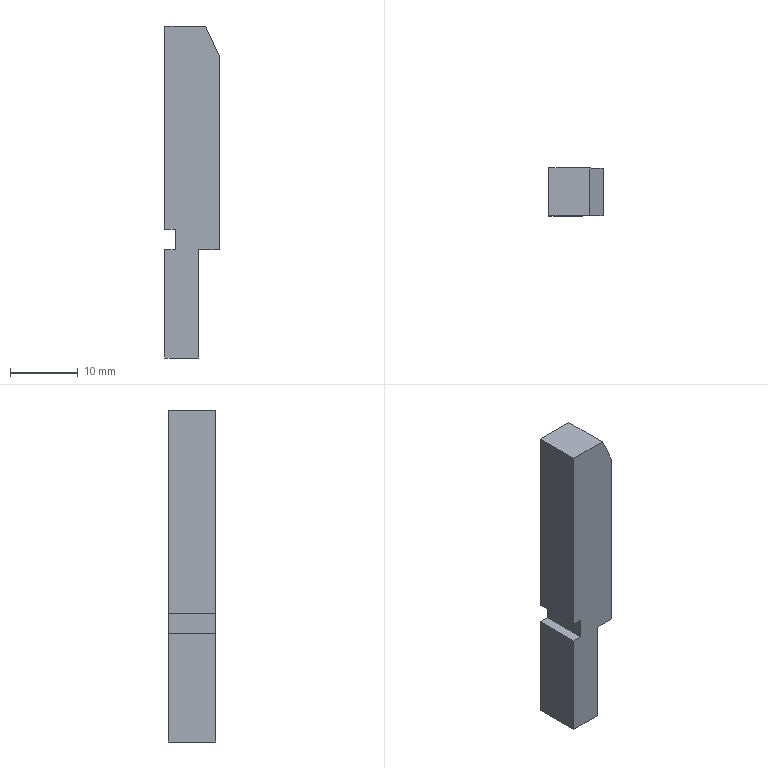Part | STEP file | Riveting product locating pin | 1 solid | 13 faces | box 8 x 7 x 49 mm | volume 2346 mm3 | plane 13
STEP:
#1=CARTESIAN_POINT('',(0.,0.,0.));
#2=DIRECTION('',(0.,0.,1.));
#3=DIRECTION('',(1.,0.,0.));
#4=AXIS2_PLACEMENT_3D('',#1,#2,#3);
#5=CARTESIAN_POINT('',(0.,8.,49.));
#6=VERTEX_POINT('',#5);
#7=CARTESIAN_POINT('',(0.,8.,19.));
#8=VERTEX_POINT('',#7);
#9=CARTESIAN_POINT('',(0.,8.,49.));
#10=DIRECTION('',(0.,0.,-1.));
#11=VECTOR('',#10,1.);
#12=LINE('',#9,#11);
#13=CARTESIAN_POINT('',(0.,0.,49.));
#14=DIRECTION('',(1.,0.,0.));
#15=DIRECTION('',(0.,0.,-1.));
#16=AXIS2_PLACEMENT_3D('',#13,#14,#15);
#17=PLANE('',#16);
#18=CARTESIAN_POINT('',(0.,8.));
#19=DIRECTION('',(1.,0.));
#20=VECTOR('',#19,1.);
#21=LINE('',#18,#20);
#22=(GEOMETRIC_REPRESENTATION_CONTEXT(2)PARAMETRIC_REPRESENTATION_CONTEXT()REPRESENTATION_CONTEXT('',''));
#23=DEFINITIONAL_REPRESENTATION('',(#21),#22);
#24=PCURVE('',#17,#23);
#25=CARTESIAN_POINT('',(0.,8.,49.));
#26=DIRECTION('',(0.,-1.,0.));
#27=DIRECTION('',(0.,0.,-1.));
#28=AXIS2_PLACEMENT_3D('',#25,#26,#27);
#29=PLANE('',#28);
#30=CARTESIAN_POINT('',(0.,0.));
#31=DIRECTION('',(1.,0.));
#32=VECTOR('',#31,1.);
#33=LINE('',#30,#32);
#34=(GEOMETRIC_REPRESENTATION_CONTEXT(2)PARAMETRIC_REPRESENTATION_CONTEXT()REPRESENTATION_CONTEXT('',''));
#35=DEFINITIONAL_REPRESENTATION('',(#33),#34);
#36=PCURVE('',#29,#35);
#37=SURFACE_CURVE('',#12,(#24,#36),.PCURVE_S1.);
#38=EDGE_CURVE('',#6,#8,#37,.T.);
#39=ORIENTED_EDGE('',*,*,#38,.T.);
#40=CARTESIAN_POINT('',(0.,1.,19.));
#41=VERTEX_POINT('',#40);
#42=CARTESIAN_POINT('',(0.,15.846,19.));
#43=DIRECTION('',(0.,1.,0.));
#44=VECTOR('',#43,1.);
#45=LINE('',#42,#44);
#46=CARTESIAN_POINT('',(30.,15.846));
#47=DIRECTION('',(0.,1.));
#48=VECTOR('',#47,1.);
#49=LINE('',#46,#48);
#50=(GEOMETRIC_REPRESENTATION_CONTEXT(2)PARAMETRIC_REPRESENTATION_CONTEXT()REPRESENTATION_CONTEXT('',''));
#51=DEFINITIONAL_REPRESENTATION('',(#49),#50);
#52=PCURVE('',#17,#51);
#53=CARTESIAN_POINT('',(1.5,15.846,19.));
#54=DIRECTION('',(0.,0.,1.));
#55=DIRECTION('',(0.,-1.,0.));
#56=AXIS2_PLACEMENT_3D('',#53,#54,#55);
#57=PLANE('',#56);
#58=CARTESIAN_POINT('',(0.,-1.5));
#59=DIRECTION('',(-1.,0.));
#60=VECTOR('',#59,1.);
#61=LINE('',#58,#60);
#62=(GEOMETRIC_REPRESENTATION_CONTEXT(2)PARAMETRIC_REPRESENTATION_CONTEXT()REPRESENTATION_CONTEXT('',''));
#63=DEFINITIONAL_REPRESENTATION('',(#61),#62);
#64=PCURVE('',#57,#63);
#65=SURFACE_CURVE('',#45,(#52,#64),.PCURVE_S1.);
#66=EDGE_CURVE('',#41,#8,#65,.T.);
#67=ORIENTED_EDGE('',*,*,#66,.F.);
#68=CARTESIAN_POINT('',(0.,1.,49.));
#69=VERTEX_POINT('',#68);
#70=CARTESIAN_POINT('',(0.,1.,49.));
#71=DIRECTION('',(0.,0.,-1.));
#72=VECTOR('',#71,1.);
#73=LINE('',#70,#72);
#74=CARTESIAN_POINT('',(0.,1.));
#75=DIRECTION('',(1.,0.));
#76=VECTOR('',#75,1.);
#77=LINE('',#74,#76);
#78=(GEOMETRIC_REPRESENTATION_CONTEXT(2)PARAMETRIC_REPRESENTATION_CONTEXT()REPRESENTATION_CONTEXT('',''));
#79=DEFINITIONAL_REPRESENTATION('',(#77),#78);
#80=PCURVE('',#17,#79);
#81=CARTESIAN_POINT('',(0.,1.,49.));
#82=DIRECTION('',(0.,1.,0.));
#83=DIRECTION('',(0.,0.,1.));
#84=AXIS2_PLACEMENT_3D('',#81,#82,#83);
#85=PLANE('',#84);
#86=CARTESIAN_POINT('',(0.,0.));
#87=DIRECTION('',(-1.,0.));
#88=VECTOR('',#87,1.);
#89=LINE('',#86,#88);
#90=(GEOMETRIC_REPRESENTATION_CONTEXT(2)PARAMETRIC_REPRESENTATION_CONTEXT()REPRESENTATION_CONTEXT('',''));
#91=DEFINITIONAL_REPRESENTATION('',(#89),#90);
#92=PCURVE('',#85,#91);
#93=SURFACE_CURVE('',#73,(#80,#92),.PCURVE_S1.);
#94=EDGE_CURVE('',#69,#41,#93,.T.);
#95=ORIENTED_EDGE('',*,*,#94,.F.);
#96=CARTESIAN_POINT('',(0.,0.,49.));
#97=DIRECTION('',(0.,-1.,0.));
#98=VECTOR('',#97,1.);
#99=LINE('',#96,#98);
#100=CARTESIAN_POINT('',(0.,0.));
#101=DIRECTION('',(0.,-1.));
#102=VECTOR('',#101,1.);
#103=LINE('',#100,#102);
#104=(GEOMETRIC_REPRESENTATION_CONTEXT(2)PARAMETRIC_REPRESENTATION_CONTEXT()REPRESENTATION_CONTEXT('',''));
#105=DEFINITIONAL_REPRESENTATION('',(#103),#104);
#106=PCURVE('',#17,#105);
#107=CARTESIAN_POINT('',(0.,8.,49.));
#108=DIRECTION('',(0.,0.,-1.));
#109=DIRECTION('',(-1.,0.,0.));
#110=AXIS2_PLACEMENT_3D('',#107,#108,#109);
#111=PLANE('',#110);
#112=CARTESIAN_POINT('',(0.,-8.));
#113=DIRECTION('',(0.,-1.));
#114=VECTOR('',#113,1.);
#115=LINE('',#112,#114);
#116=(GEOMETRIC_REPRESENTATION_CONTEXT(2)PARAMETRIC_REPRESENTATION_CONTEXT()REPRESENTATION_CONTEXT('',''));
#117=DEFINITIONAL_REPRESENTATION('',(#115),#116);
#118=PCURVE('',#111,#117);
#119=SURFACE_CURVE('',#99,(#106,#118),.PCURVE_S1.);
#120=EDGE_CURVE('',#6,#69,#119,.T.);
#121=ORIENTED_EDGE('',*,*,#120,.F.);
#122=EDGE_LOOP('',(#39,#67,#95,#121));
#123=FACE_BOUND('',#122,.T.);
#124=ADVANCED_FACE('',(#123),#17,.F.);
#125=CARTESIAN_POINT('',(0.,1.,16.));
#126=VERTEX_POINT('',#125);
#127=CARTESIAN_POINT('',(0.,1.,0.));
#128=VERTEX_POINT('',#127);
#129=CARTESIAN_POINT('',(0.,1.,49.));
#130=DIRECTION('',(0.,0.,-1.));
#131=VECTOR('',#130,1.);
#132=LINE('',#129,#131);
#133=CARTESIAN_POINT('',(0.,0.,49.));
#134=DIRECTION('',(1.,0.,0.));
#135=DIRECTION('',(0.,0.,-1.));
#136=AXIS2_PLACEMENT_3D('',#133,#134,#135);
#137=PLANE('',#136);
#138=CARTESIAN_POINT('',(0.,1.));
#139=DIRECTION('',(1.,0.));
#140=VECTOR('',#139,1.);
#141=LINE('',#138,#140);
#142=(GEOMETRIC_REPRESENTATION_CONTEXT(2)PARAMETRIC_REPRESENTATION_CONTEXT()REPRESENTATION_CONTEXT('',''));
#143=DEFINITIONAL_REPRESENTATION('',(#141),#142);
#144=PCURVE('',#137,#143);
#145=CARTESIAN_POINT('',(0.,0.));
#146=DIRECTION('',(-1.,0.));
#147=VECTOR('',#146,1.);
#148=LINE('',#145,#147);
#149=(GEOMETRIC_REPRESENTATION_CONTEXT(2)PARAMETRIC_REPRESENTATION_CONTEXT()REPRESENTATION_CONTEXT('',''));
#150=DEFINITIONAL_REPRESENTATION('',(#148),#149);
#151=PCURVE('',#85,#150);
#152=SURFACE_CURVE('',#132,(#144,#151),.PCURVE_S1.);
#153=EDGE_CURVE('',#126,#128,#152,.T.);
#154=ORIENTED_EDGE('',*,*,#153,.F.);
#155=CARTESIAN_POINT('',(0.,8.,16.));
#156=VERTEX_POINT('',#155);
#157=CARTESIAN_POINT('',(0.,15.846,16.));
#158=DIRECTION('',(0.,-1.,0.));
#159=VECTOR('',#158,1.);
#160=LINE('',#157,#159);
#161=CARTESIAN_POINT('',(33.,15.846));
#162=DIRECTION('',(0.,-1.));
#163=VECTOR('',#162,1.);
#164=LINE('',#161,#163);
#165=(GEOMETRIC_REPRESENTATION_CONTEXT(2)PARAMETRIC_REPRESENTATION_CONTEXT()REPRESENTATION_CONTEXT('',''));
#166=DEFINITIONAL_REPRESENTATION('',(#164),#165);
#167=PCURVE('',#137,#166);
#168=CARTESIAN_POINT('',(1.5,15.846,16.));
#169=DIRECTION('',(0.,0.,-1.));
#170=DIRECTION('',(0.,1.,0.));
#171=AXIS2_PLACEMENT_3D('',#168,#169,#170);
#172=PLANE('',#171);
#173=CARTESIAN_POINT('',(0.,-1.5));
#174=DIRECTION('',(-1.,0.));
#175=VECTOR('',#174,1.);
#176=LINE('',#173,#175);
#177=(GEOMETRIC_REPRESENTATION_CONTEXT(2)PARAMETRIC_REPRESENTATION_CONTEXT()REPRESENTATION_CONTEXT('',''));
#178=DEFINITIONAL_REPRESENTATION('',(#176),#177);
#179=PCURVE('',#172,#178);
#180=SURFACE_CURVE('',#160,(#167,#179),.PCURVE_S1.);
#181=EDGE_CURVE('',#156,#126,#180,.T.);
#182=ORIENTED_EDGE('',*,*,#181,.F.);
#183=CARTESIAN_POINT('',(0.,8.,0.));
#184=VERTEX_POINT('',#183);
#185=CARTESIAN_POINT('',(0.,8.,49.));
#186=DIRECTION('',(0.,0.,-1.));
#187=VECTOR('',#186,1.);
#188=LINE('',#185,#187);
#189=CARTESIAN_POINT('',(0.,8.));
#190=DIRECTION('',(1.,0.));
#191=VECTOR('',#190,1.);
#192=LINE('',#189,#191);
#193=(GEOMETRIC_REPRESENTATION_CONTEXT(2)PARAMETRIC_REPRESENTATION_CONTEXT()REPRESENTATION_CONTEXT('',''));
#194=DEFINITIONAL_REPRESENTATION('',(#192),#193);
#195=PCURVE('',#137,#194);
#196=CARTESIAN_POINT('',(0.,0.));
#197=DIRECTION('',(1.,0.));
#198=VECTOR('',#197,1.);
#199=LINE('',#196,#198);
#200=(GEOMETRIC_REPRESENTATION_CONTEXT(2)PARAMETRIC_REPRESENTATION_CONTEXT()REPRESENTATION_CONTEXT('',''));
#201=DEFINITIONAL_REPRESENTATION('',(#199),#200);
#202=PCURVE('',#29,#201);
#203=SURFACE_CURVE('',#188,(#195,#202),.PCURVE_S1.);
#204=EDGE_CURVE('',#156,#184,#203,.T.);
#205=ORIENTED_EDGE('',*,*,#204,.T.);
#206=CARTESIAN_POINT('',(0.,0.,0.));
#207=DIRECTION('',(0.,-1.,0.));
#208=VECTOR('',#207,1.);
#209=LINE('',#206,#208);
#210=CARTESIAN_POINT('',(49.,0.));
#211=DIRECTION('',(0.,-1.));
#212=VECTOR('',#211,1.);
#213=LINE('',#210,#212);
#214=(GEOMETRIC_REPRESENTATION_CONTEXT(2)PARAMETRIC_REPRESENTATION_CONTEXT()REPRESENTATION_CONTEXT('',''));
#215=DEFINITIONAL_REPRESENTATION('',(#213),#214);
#216=PCURVE('',#137,#215);
#217=CARTESIAN_POINT('',(0.,8.,0.));
#218=DIRECTION('',(0.,0.,-1.));
#219=DIRECTION('',(-1.,0.,0.));
#220=AXIS2_PLACEMENT_3D('',#217,#218,#219);
#221=PLANE('',#220);
#222=CARTESIAN_POINT('',(0.,-8.));
#223=DIRECTION('',(0.,-1.));
#224=VECTOR('',#223,1.);
#225=LINE('',#222,#224);
#226=(GEOMETRIC_REPRESENTATION_CONTEXT(2)PARAMETRIC_REPRESENTATION_CONTEXT()REPRESENTATION_CONTEXT('',''));
#227=DEFINITIONAL_REPRESENTATION('',(#225),#226);
#228=PCURVE('',#221,#227);
#229=SURFACE_CURVE('',#209,(#216,#228),.PCURVE_S1.);
#230=EDGE_CURVE('',#184,#128,#229,.T.);
#231=ORIENTED_EDGE('',*,*,#230,.T.);
#232=EDGE_LOOP('',(#154,#182,#205,#231));
#233=FACE_BOUND('',#232,.T.);
#234=ADVANCED_FACE('',(#233),#137,.F.);
#235=CARTESIAN_POINT('',(8.,1.,44.711));
#236=VERTEX_POINT('',#235);
#237=CARTESIAN_POINT('',(8.,1.,16.));
#238=VERTEX_POINT('',#237);
#239=CARTESIAN_POINT('',(8.,1.,49.));
#240=DIRECTION('',(0.,0.,-1.));
#241=VECTOR('',#240,1.);
#242=LINE('',#239,#241);
#243=CARTESIAN_POINT('',(0.,8.));
#244=DIRECTION('',(-1.,0.));
#245=VECTOR('',#244,1.);
#246=LINE('',#243,#245);
#247=(GEOMETRIC_REPRESENTATION_CONTEXT(2)PARAMETRIC_REPRESENTATION_CONTEXT()REPRESENTATION_CONTEXT('',''));
#248=DEFINITIONAL_REPRESENTATION('',(#246),#247);
#249=PCURVE('',#85,#248);
#250=CARTESIAN_POINT('',(8.,0.,49.));
#251=DIRECTION('',(-1.,0.,0.));
#252=DIRECTION('',(0.,0.,1.));
#253=AXIS2_PLACEMENT_3D('',#250,#251,#252);
#254=PLANE('',#253);
#255=CARTESIAN_POINT('',(0.,1.));
#256=DIRECTION('',(-1.,0.));
#257=VECTOR('',#256,1.);
#258=LINE('',#255,#257);
#259=(GEOMETRIC_REPRESENTATION_CONTEXT(2)PARAMETRIC_REPRESENTATION_CONTEXT()REPRESENTATION_CONTEXT('',''));
#260=DEFINITIONAL_REPRESENTATION('',(#258),#259);
#261=PCURVE('',#254,#260);
#262=SURFACE_CURVE('',#242,(#249,#261),.PCURVE_S1.);
#263=EDGE_CURVE('',#236,#238,#262,.T.);
#264=ORIENTED_EDGE('',*,*,#263,.F.);
#265=CARTESIAN_POINT('',(6.,1.,49.));
#266=VERTEX_POINT('',#265);
#267=CARTESIAN_POINT('',(6.,1.,49.));
#268=DIRECTION('',(-0.4226,0.,0.9063));
#269=VECTOR('',#268,1.);
#270=LINE('',#267,#269);
#271=CARTESIAN_POINT('',(0.,6.));
#272=DIRECTION('',(0.9063,-0.4226));
#273=VECTOR('',#272,1.);
#274=LINE('',#271,#273);
#275=(GEOMETRIC_REPRESENTATION_CONTEXT(2)PARAMETRIC_REPRESENTATION_CONTEXT()REPRESENTATION_CONTEXT('',''));
#276=DEFINITIONAL_REPRESENTATION('',(#274),#275);
#277=PCURVE('',#85,#276);
#278=CARTESIAN_POINT('',(6.,8.,49.));
#279=DIRECTION('',(-0.9063,0.,-0.4226));
#280=DIRECTION('',(-0.4226,0.,0.9063));
#281=AXIS2_PLACEMENT_3D('',#278,#279,#280);
#282=PLANE('',#281);
#283=CARTESIAN_POINT('',(0.,-7.));
#284=DIRECTION('',(1.,0.));
#285=VECTOR('',#284,1.);
#286=LINE('',#283,#285);
#287=(GEOMETRIC_REPRESENTATION_CONTEXT(2)PARAMETRIC_REPRESENTATION_CONTEXT()REPRESENTATION_CONTEXT('',''));
#288=DEFINITIONAL_REPRESENTATION('',(#286),#287);
#289=PCURVE('',#282,#288);
#290=SURFACE_CURVE('',#270,(#277,#289),.PCURVE_S1.);
#291=EDGE_CURVE('',#236,#266,#290,.T.);
#292=ORIENTED_EDGE('',*,*,#291,.T.);
#293=CARTESIAN_POINT('',(0.,1.,49.));
#294=DIRECTION('',(1.,0.,0.));
#295=VECTOR('',#294,1.);
#296=LINE('',#293,#295);
#297=CARTESIAN_POINT('',(0.,0.));
#298=DIRECTION('',(0.,1.));
#299=VECTOR('',#298,1.);
#300=LINE('',#297,#299);
#301=(GEOMETRIC_REPRESENTATION_CONTEXT(2)PARAMETRIC_REPRESENTATION_CONTEXT()REPRESENTATION_CONTEXT('',''));
#302=DEFINITIONAL_REPRESENTATION('',(#300),#301);
#303=PCURVE('',#85,#302);
#304=CARTESIAN_POINT('',(0.,-7.));
#305=DIRECTION('',(-1.,0.));
#306=VECTOR('',#305,1.);
#307=LINE('',#304,#306);
#308=(GEOMETRIC_REPRESENTATION_CONTEXT(2)PARAMETRIC_REPRESENTATION_CONTEXT()REPRESENTATION_CONTEXT('',''));
#309=DEFINITIONAL_REPRESENTATION('',(#307),#308);
#310=PCURVE('',#111,#309);
#311=SURFACE_CURVE('',#296,(#303,#310),.PCURVE_S1.);
#312=EDGE_CURVE('',#69,#266,#311,.T.);
#313=ORIENTED_EDGE('',*,*,#312,.F.);
#314=ORIENTED_EDGE('',*,*,#94,.T.);
#315=CARTESIAN_POINT('',(1.5,1.,19.));
#316=VERTEX_POINT('',#315);
#317=CARTESIAN_POINT('',(0.,1.,19.));
#318=DIRECTION('',(1.,0.,0.));
#319=VECTOR('',#318,1.);
#320=LINE('',#317,#319);
#321=CARTESIAN_POINT('',(-30.,0.));
#322=DIRECTION('',(0.,1.));
#323=VECTOR('',#322,1.);
#324=LINE('',#321,#323);
#325=(GEOMETRIC_REPRESENTATION_CONTEXT(2)PARAMETRIC_REPRESENTATION_CONTEXT()REPRESENTATION_CONTEXT('',''));
#326=DEFINITIONAL_REPRESENTATION('',(#324),#325);
#327=PCURVE('',#85,#326);
#328=CARTESIAN_POINT('',(14.846,-1.5));
#329=DIRECTION('',(0.,1.));
#330=VECTOR('',#329,1.);
#331=LINE('',#328,#330);
#332=(GEOMETRIC_REPRESENTATION_CONTEXT(2)PARAMETRIC_REPRESENTATION_CONTEXT()REPRESENTATION_CONTEXT('',''));
#333=DEFINITIONAL_REPRESENTATION('',(#331),#332);
#334=PCURVE('',#57,#333);
#335=SURFACE_CURVE('',#320,(#327,#334),.PCURVE_S1.);
#336=EDGE_CURVE('',#41,#316,#335,.T.);
#337=ORIENTED_EDGE('',*,*,#336,.T.);
#338=CARTESIAN_POINT('',(1.5,1.,16.));
#339=VERTEX_POINT('',#338);
#340=CARTESIAN_POINT('',(1.5,1.,49.));
#341=DIRECTION('',(0.,0.,-1.));
#342=VECTOR('',#341,1.);
#343=LINE('',#340,#342);
#344=CARTESIAN_POINT('',(0.,1.5));
#345=DIRECTION('',(-1.,0.));
#346=VECTOR('',#345,1.);
#347=LINE('',#344,#346);
#348=(GEOMETRIC_REPRESENTATION_CONTEXT(2)PARAMETRIC_REPRESENTATION_CONTEXT()REPRESENTATION_CONTEXT('',''));
#349=DEFINITIONAL_REPRESENTATION('',(#347),#348);
#350=PCURVE('',#85,#349);
#351=CARTESIAN_POINT('',(1.5,-3.859,19.));
#352=DIRECTION('',(1.,0.,0.));
#353=DIRECTION('',(0.,0.,-1.));
#354=AXIS2_PLACEMENT_3D('',#351,#352,#353);
#355=PLANE('',#354);
#356=CARTESIAN_POINT('',(-30.,4.859));
#357=DIRECTION('',(1.,0.));
#358=VECTOR('',#357,1.);
#359=LINE('',#356,#358);
#360=(GEOMETRIC_REPRESENTATION_CONTEXT(2)PARAMETRIC_REPRESENTATION_CONTEXT()REPRESENTATION_CONTEXT('',''));
#361=DEFINITIONAL_REPRESENTATION('',(#359),#360);
#362=PCURVE('',#355,#361);
#363=SURFACE_CURVE('',#343,(#350,#362),.PCURVE_S1.);
#364=EDGE_CURVE('',#316,#339,#363,.T.);
#365=ORIENTED_EDGE('',*,*,#364,.T.);
#366=CARTESIAN_POINT('',(0.,1.,16.));
#367=DIRECTION('',(-1.,0.,0.));
#368=VECTOR('',#367,1.);
#369=LINE('',#366,#368);
#370=CARTESIAN_POINT('',(-33.,0.));
#371=DIRECTION('',(0.,-1.));
#372=VECTOR('',#371,1.);
#373=LINE('',#370,#372);
#374=(GEOMETRIC_REPRESENTATION_CONTEXT(2)PARAMETRIC_REPRESENTATION_CONTEXT()REPRESENTATION_CONTEXT('',''));
#375=DEFINITIONAL_REPRESENTATION('',(#373),#374);
#376=PCURVE('',#85,#375);
#377=CARTESIAN_POINT('',(-14.846,-1.5));
#378=DIRECTION('',(0.,-1.));
#379=VECTOR('',#378,1.);
#380=LINE('',#377,#379);
#381=(GEOMETRIC_REPRESENTATION_CONTEXT(2)PARAMETRIC_REPRESENTATION_CONTEXT()REPRESENTATION_CONTEXT('',''));
#382=DEFINITIONAL_REPRESENTATION('',(#380),#381);
#383=PCURVE('',#172,#382);
#384=SURFACE_CURVE('',#369,(#376,#383),.PCURVE_S1.);
#385=EDGE_CURVE('',#339,#126,#384,.T.);
#386=ORIENTED_EDGE('',*,*,#385,.T.);
#387=ORIENTED_EDGE('',*,*,#153,.T.);
#388=CARTESIAN_POINT('',(5.,1.,0.));
#389=VERTEX_POINT('',#388);
#390=CARTESIAN_POINT('',(0.,1.,0.));
#391=DIRECTION('',(1.,0.,0.));
#392=VECTOR('',#391,1.);
#393=LINE('',#390,#392);
#394=CARTESIAN_POINT('',(-49.,0.));
#395=DIRECTION('',(0.,1.));
#396=VECTOR('',#395,1.);
#397=LINE('',#394,#396);
#398=(GEOMETRIC_REPRESENTATION_CONTEXT(2)PARAMETRIC_REPRESENTATION_CONTEXT()REPRESENTATION_CONTEXT('',''));
#399=DEFINITIONAL_REPRESENTATION('',(#397),#398);
#400=PCURVE('',#85,#399);
#401=CARTESIAN_POINT('',(0.,-7.));
#402=DIRECTION('',(-1.,0.));
#403=VECTOR('',#402,1.);
#404=LINE('',#401,#403);
#405=(GEOMETRIC_REPRESENTATION_CONTEXT(2)PARAMETRIC_REPRESENTATION_CONTEXT()REPRESENTATION_CONTEXT('',''));
#406=DEFINITIONAL_REPRESENTATION('',(#404),#405);
#407=PCURVE('',#221,#406);
#408=SURFACE_CURVE('',#393,(#400,#407),.PCURVE_S1.);
#409=EDGE_CURVE('',#128,#389,#408,.T.);
#410=ORIENTED_EDGE('',*,*,#409,.T.);
#411=CARTESIAN_POINT('',(5.,1.,16.));
#412=VERTEX_POINT('',#411);
#413=CARTESIAN_POINT('',(5.,1.,49.));
#414=DIRECTION('',(0.,0.,1.));
#415=VECTOR('',#414,1.);
#416=LINE('',#413,#415);
#417=CARTESIAN_POINT('',(0.,5.));
#418=DIRECTION('',(1.,0.));
#419=VECTOR('',#418,1.);
#420=LINE('',#417,#419);
#421=(GEOMETRIC_REPRESENTATION_CONTEXT(2)PARAMETRIC_REPRESENTATION_CONTEXT()REPRESENTATION_CONTEXT('',''));
#422=DEFINITIONAL_REPRESENTATION('',(#420),#421);
#423=PCURVE('',#85,#422);
#424=CARTESIAN_POINT('',(5.,9.859,16.));
#425=DIRECTION('',(-1.,0.,0.));
#426=DIRECTION('',(0.,-1.,0.));
#427=AXIS2_PLACEMENT_3D('',#424,#425,#426);
#428=PLANE('',#427);
#429=CARTESIAN_POINT('',(8.859,33.));
#430=DIRECTION('',(0.,1.));
#431=VECTOR('',#430,1.);
#432=LINE('',#429,#431);
#433=(GEOMETRIC_REPRESENTATION_CONTEXT(2)PARAMETRIC_REPRESENTATION_CONTEXT()REPRESENTATION_CONTEXT('',''));
#434=DEFINITIONAL_REPRESENTATION('',(#432),#433);
#435=PCURVE('',#428,#434);
#436=SURFACE_CURVE('',#416,(#423,#435),.PCURVE_S1.);
#437=EDGE_CURVE('',#389,#412,#436,.T.);
#438=ORIENTED_EDGE('',*,*,#437,.T.);
#439=CARTESIAN_POINT('',(0.,1.,16.));
#440=DIRECTION('',(1.,0.,0.));
#441=VECTOR('',#440,1.);
#442=LINE('',#439,#441);
#443=CARTESIAN_POINT('',(-33.,0.));
#444=DIRECTION('',(0.,1.));
#445=VECTOR('',#444,1.);
#446=LINE('',#443,#445);
#447=(GEOMETRIC_REPRESENTATION_CONTEXT(2)PARAMETRIC_REPRESENTATION_CONTEXT()REPRESENTATION_CONTEXT('',''));
#448=DEFINITIONAL_REPRESENTATION('',(#446),#447);
#449=PCURVE('',#85,#448);
#450=CARTESIAN_POINT('',(5.,-2.91,16.));
#451=DIRECTION('',(0.,0.,1.));
#452=DIRECTION('',(1.,0.,0.));
#453=AXIS2_PLACEMENT_3D('',#450,#451,#452);
#454=PLANE('',#453);
#455=CARTESIAN_POINT('',(-5.,3.91));
#456=DIRECTION('',(1.,0.));
#457=VECTOR('',#456,1.);
#458=LINE('',#455,#457);
#459=(GEOMETRIC_REPRESENTATION_CONTEXT(2)PARAMETRIC_REPRESENTATION_CONTEXT()REPRESENTATION_CONTEXT('',''));
#460=DEFINITIONAL_REPRESENTATION('',(#458),#459);
#461=PCURVE('',#454,#460);
#462=SURFACE_CURVE('',#442,(#449,#461),.PCURVE_S1.);
#463=EDGE_CURVE('',#412,#238,#462,.T.);
#464=ORIENTED_EDGE('',*,*,#463,.T.);
#465=EDGE_LOOP('',(#264,#292,#313,#314,#337,#365,#386,#387,#410,#438,#464));
#466=FACE_BOUND('',#465,.T.);
#467=ADVANCED_FACE('',(#466),#85,.F.);
#468=CARTESIAN_POINT('',(8.,8.,44.711));
#469=VERTEX_POINT('',#468);
#470=CARTESIAN_POINT('',(8.,8.,16.));
#471=VERTEX_POINT('',#470);
#472=CARTESIAN_POINT('',(8.,8.,49.));
#473=DIRECTION('',(0.,0.,-1.));
#474=VECTOR('',#473,1.);
#475=LINE('',#472,#474);
#476=CARTESIAN_POINT('',(0.,8.));
#477=DIRECTION('',(-1.,0.));
#478=VECTOR('',#477,1.);
#479=LINE('',#476,#478);
#480=(GEOMETRIC_REPRESENTATION_CONTEXT(2)PARAMETRIC_REPRESENTATION_CONTEXT()REPRESENTATION_CONTEXT('',''));
#481=DEFINITIONAL_REPRESENTATION('',(#479),#480);
#482=PCURVE('',#254,#481);
#483=CARTESIAN_POINT('',(0.,8.));
#484=DIRECTION('',(1.,0.));
#485=VECTOR('',#484,1.);
#486=LINE('',#483,#485);
#487=(GEOMETRIC_REPRESENTATION_CONTEXT(2)PARAMETRIC_REPRESENTATION_CONTEXT()REPRESENTATION_CONTEXT('',''));
#488=DEFINITIONAL_REPRESENTATION('',(#486),#487);
#489=PCURVE('',#29,#488);
#490=SURFACE_CURVE('',#475,(#482,#489),.PCURVE_S1.);
#491=EDGE_CURVE('',#469,#471,#490,.T.);
#492=ORIENTED_EDGE('',*,*,#491,.F.);
#493=CARTESIAN_POINT('',(8.,0.,44.711));
#494=DIRECTION('',(0.,-1.,0.));
#495=VECTOR('',#494,1.);
#496=LINE('',#493,#495);
#497=CARTESIAN_POINT('',(-4.289,0.));
#498=DIRECTION('',(0.,-1.));
#499=VECTOR('',#498,1.);
#500=LINE('',#497,#499);
#501=(GEOMETRIC_REPRESENTATION_CONTEXT(2)PARAMETRIC_REPRESENTATION_CONTEXT()REPRESENTATION_CONTEXT('',''));
#502=DEFINITIONAL_REPRESENTATION('',(#500),#501);
#503=PCURVE('',#254,#502);
#504=CARTESIAN_POINT('',(-4.732,-8.));
#505=DIRECTION('',(0.,-1.));
#506=VECTOR('',#505,1.);
#507=LINE('',#504,#506);
#508=(GEOMETRIC_REPRESENTATION_CONTEXT(2)PARAMETRIC_REPRESENTATION_CONTEXT()REPRESENTATION_CONTEXT('',''));
#509=DEFINITIONAL_REPRESENTATION('',(#507),#508);
#510=PCURVE('',#282,#509);
#511=SURFACE_CURVE('',#496,(#503,#510),.PCURVE_S1.);
#512=EDGE_CURVE('',#469,#236,#511,.T.);
#513=ORIENTED_EDGE('',*,*,#512,.T.);
#514=ORIENTED_EDGE('',*,*,#263,.T.);
#515=CARTESIAN_POINT('',(8.,0.,16.));
#516=DIRECTION('',(0.,1.,0.));
#517=VECTOR('',#516,1.);
#518=LINE('',#515,#517);
#519=CARTESIAN_POINT('',(-33.,0.));
#520=DIRECTION('',(0.,1.));
#521=VECTOR('',#520,1.);
#522=LINE('',#519,#521);
#523=(GEOMETRIC_REPRESENTATION_CONTEXT(2)PARAMETRIC_REPRESENTATION_CONTEXT()REPRESENTATION_CONTEXT('',''));
#524=DEFINITIONAL_REPRESENTATION('',(#522),#523);
#525=PCURVE('',#254,#524);
#526=CARTESIAN_POINT('',(3.,2.91));
#527=DIRECTION('',(0.,1.));
#528=VECTOR('',#527,1.);
#529=LINE('',#526,#528);
#530=(GEOMETRIC_REPRESENTATION_CONTEXT(2)PARAMETRIC_REPRESENTATION_CONTEXT()REPRESENTATION_CONTEXT('',''));
#531=DEFINITIONAL_REPRESENTATION('',(#529),#530);
#532=PCURVE('',#454,#531);
#533=SURFACE_CURVE('',#518,(#525,#532),.PCURVE_S1.);
#534=EDGE_CURVE('',#238,#471,#533,.T.);
#535=ORIENTED_EDGE('',*,*,#534,.T.);
#536=EDGE_LOOP('',(#492,#513,#514,#535));
#537=FACE_BOUND('',#536,.T.);
#538=ADVANCED_FACE('',(#537),#254,.F.);
#539=CARTESIAN_POINT('',(6.,8.,49.));
#540=VERTEX_POINT('',#539);
#541=CARTESIAN_POINT('',(0.,8.,49.));
#542=DIRECTION('',(-1.,0.,0.));
#543=VECTOR('',#542,1.);
#544=LINE('',#541,#543);
#545=CARTESIAN_POINT('',(0.,0.));
#546=DIRECTION('',(0.,-1.));
#547=VECTOR('',#546,1.);
#548=LINE('',#545,#547);
#549=(GEOMETRIC_REPRESENTATION_CONTEXT(2)PARAMETRIC_REPRESENTATION_CONTEXT()REPRESENTATION_CONTEXT('',''));
#550=DEFINITIONAL_REPRESENTATION('',(#548),#549);
#551=PCURVE('',#29,#550);
#552=CARTESIAN_POINT('',(0.,0.));
#553=DIRECTION('',(1.,0.));
#554=VECTOR('',#553,1.);
#555=LINE('',#552,#554);
#556=(GEOMETRIC_REPRESENTATION_CONTEXT(2)PARAMETRIC_REPRESENTATION_CONTEXT()REPRESENTATION_CONTEXT('',''));
#557=DEFINITIONAL_REPRESENTATION('',(#555),#556);
#558=PCURVE('',#111,#557);
#559=SURFACE_CURVE('',#544,(#551,#558),.PCURVE_S1.);
#560=EDGE_CURVE('',#540,#6,#559,.T.);
#561=ORIENTED_EDGE('',*,*,#560,.F.);
#562=CARTESIAN_POINT('',(6.,8.,49.));
#563=DIRECTION('',(0.4226,0.,-0.9063));
#564=VECTOR('',#563,1.);
#565=LINE('',#562,#564);
#566=CARTESIAN_POINT('',(0.,6.));
#567=DIRECTION('',(0.9063,0.4226));
#568=VECTOR('',#567,1.);
#569=LINE('',#566,#568);
#570=(GEOMETRIC_REPRESENTATION_CONTEXT(2)PARAMETRIC_REPRESENTATION_CONTEXT()REPRESENTATION_CONTEXT('',''));
#571=DEFINITIONAL_REPRESENTATION('',(#569),#570);
#572=PCURVE('',#29,#571);
#573=CARTESIAN_POINT('',(0.,0.));
#574=DIRECTION('',(-1.,0.));
#575=VECTOR('',#574,1.);
#576=LINE('',#573,#575);
#577=(GEOMETRIC_REPRESENTATION_CONTEXT(2)PARAMETRIC_REPRESENTATION_CONTEXT()REPRESENTATION_CONTEXT('',''));
#578=DEFINITIONAL_REPRESENTATION('',(#576),#577);
#579=PCURVE('',#282,#578);
#580=SURFACE_CURVE('',#565,(#572,#579),.PCURVE_S1.);
#581=EDGE_CURVE('',#540,#469,#580,.T.);
#582=ORIENTED_EDGE('',*,*,#581,.T.);
#583=ORIENTED_EDGE('',*,*,#491,.T.);
#584=CARTESIAN_POINT('',(5.,8.,16.));
#585=VERTEX_POINT('',#584);
#586=CARTESIAN_POINT('',(0.,8.,16.));
#587=DIRECTION('',(-1.,0.,0.));
#588=VECTOR('',#587,1.);
#589=LINE('',#586,#588);
#590=CARTESIAN_POINT('',(33.,0.));
#591=DIRECTION('',(0.,-1.));
#592=VECTOR('',#591,1.);
#593=LINE('',#590,#592);
#594=(GEOMETRIC_REPRESENTATION_CONTEXT(2)PARAMETRIC_REPRESENTATION_CONTEXT()REPRESENTATION_CONTEXT('',''));
#595=DEFINITIONAL_REPRESENTATION('',(#593),#594);
#596=PCURVE('',#29,#595);
#597=CARTESIAN_POINT('',(-5.,10.91));
#598=DIRECTION('',(-1.,0.));
#599=VECTOR('',#598,1.);
#600=LINE('',#597,#599);
#601=(GEOMETRIC_REPRESENTATION_CONTEXT(2)PARAMETRIC_REPRESENTATION_CONTEXT()REPRESENTATION_CONTEXT('',''));
#602=DEFINITIONAL_REPRESENTATION('',(#600),#601);
#603=PCURVE('',#454,#602);
#604=SURFACE_CURVE('',#589,(#596,#603),.PCURVE_S1.);
#605=EDGE_CURVE('',#471,#585,#604,.T.);
#606=ORIENTED_EDGE('',*,*,#605,.T.);
#607=CARTESIAN_POINT('',(5.,8.,0.));
#608=VERTEX_POINT('',#607);
#609=CARTESIAN_POINT('',(5.,8.,49.));
#610=DIRECTION('',(0.,0.,-1.));
#611=VECTOR('',#610,1.);
#612=LINE('',#609,#611);
#613=CARTESIAN_POINT('',(0.,5.));
#614=DIRECTION('',(1.,0.));
#615=VECTOR('',#614,1.);
#616=LINE('',#613,#615);
#617=(GEOMETRIC_REPRESENTATION_CONTEXT(2)PARAMETRIC_REPRESENTATION_CONTEXT()REPRESENTATION_CONTEXT('',''));
#618=DEFINITIONAL_REPRESENTATION('',(#616),#617);
#619=PCURVE('',#29,#618);
#620=CARTESIAN_POINT('',(1.859,33.));
#621=DIRECTION('',(0.,-1.));
#622=VECTOR('',#621,1.);
#623=LINE('',#620,#622);
#624=(GEOMETRIC_REPRESENTATION_CONTEXT(2)PARAMETRIC_REPRESENTATION_CONTEXT()REPRESENTATION_CONTEXT('',''));
#625=DEFINITIONAL_REPRESENTATION('',(#623),#624);
#626=PCURVE('',#428,#625);
#627=SURFACE_CURVE('',#612,(#619,#626),.PCURVE_S1.);
#628=EDGE_CURVE('',#585,#608,#627,.T.);
#629=ORIENTED_EDGE('',*,*,#628,.T.);
#630=CARTESIAN_POINT('',(0.,8.,0.));
#631=DIRECTION('',(-1.,0.,0.));
#632=VECTOR('',#631,1.);
#633=LINE('',#630,#632);
#634=CARTESIAN_POINT('',(49.,0.));
#635=DIRECTION('',(0.,-1.));
#636=VECTOR('',#635,1.);
#637=LINE('',#634,#636);
#638=(GEOMETRIC_REPRESENTATION_CONTEXT(2)PARAMETRIC_REPRESENTATION_CONTEXT()REPRESENTATION_CONTEXT('',''));
#639=DEFINITIONAL_REPRESENTATION('',(#637),#638);
#640=PCURVE('',#29,#639);
#641=CARTESIAN_POINT('',(0.,0.));
#642=DIRECTION('',(1.,0.));
#643=VECTOR('',#642,1.);
#644=LINE('',#641,#643);
#645=(GEOMETRIC_REPRESENTATION_CONTEXT(2)PARAMETRIC_REPRESENTATION_CONTEXT()REPRESENTATION_CONTEXT('',''));
#646=DEFINITIONAL_REPRESENTATION('',(#644),#645);
#647=PCURVE('',#221,#646);
#648=SURFACE_CURVE('',#633,(#640,#647),.PCURVE_S1.);
#649=EDGE_CURVE('',#608,#184,#648,.T.);
#650=ORIENTED_EDGE('',*,*,#649,.T.);
#651=ORIENTED_EDGE('',*,*,#204,.F.);
#652=CARTESIAN_POINT('',(1.5,8.,16.));
#653=VERTEX_POINT('',#652);
#654=CARTESIAN_POINT('',(0.,8.,16.));
#655=DIRECTION('',(1.,0.,0.));
#656=VECTOR('',#655,1.);
#657=LINE('',#654,#656);
#658=CARTESIAN_POINT('',(33.,0.));
#659=DIRECTION('',(0.,1.));
#660=VECTOR('',#659,1.);
#661=LINE('',#658,#660);
#662=(GEOMETRIC_REPRESENTATION_CONTEXT(2)PARAMETRIC_REPRESENTATION_CONTEXT()REPRESENTATION_CONTEXT('',''));
#663=DEFINITIONAL_REPRESENTATION('',(#661),#662);
#664=PCURVE('',#29,#663);
#665=CARTESIAN_POINT('',(-7.846,-1.5));
#666=DIRECTION('',(0.,1.));
#667=VECTOR('',#666,1.);
#668=LINE('',#665,#667);
#669=(GEOMETRIC_REPRESENTATION_CONTEXT(2)PARAMETRIC_REPRESENTATION_CONTEXT()REPRESENTATION_CONTEXT('',''));
#670=DEFINITIONAL_REPRESENTATION('',(#668),#669);
#671=PCURVE('',#172,#670);
#672=SURFACE_CURVE('',#657,(#664,#671),.PCURVE_S1.);
#673=EDGE_CURVE('',#156,#653,#672,.T.);
#674=ORIENTED_EDGE('',*,*,#673,.T.);
#675=CARTESIAN_POINT('',(1.5,8.,19.));
#676=VERTEX_POINT('',#675);
#677=CARTESIAN_POINT('',(1.5,8.,49.));
#678=DIRECTION('',(0.,0.,1.));
#679=VECTOR('',#678,1.);
#680=LINE('',#677,#679);
#681=CARTESIAN_POINT('',(0.,1.5));
#682=DIRECTION('',(-1.,0.));
#683=VECTOR('',#682,1.);
#684=LINE('',#681,#683);
#685=(GEOMETRIC_REPRESENTATION_CONTEXT(2)PARAMETRIC_REPRESENTATION_CONTEXT()REPRESENTATION_CONTEXT('',''));
#686=DEFINITIONAL_REPRESENTATION('',(#684),#685);
#687=PCURVE('',#29,#686);
#688=CARTESIAN_POINT('',(-30.,11.859));
#689=DIRECTION('',(-1.,0.));
#690=VECTOR('',#689,1.);
#691=LINE('',#688,#690);
#692=(GEOMETRIC_REPRESENTATION_CONTEXT(2)PARAMETRIC_REPRESENTATION_CONTEXT()REPRESENTATION_CONTEXT('',''));
#693=DEFINITIONAL_REPRESENTATION('',(#691),#692);
#694=PCURVE('',#355,#693);
#695=SURFACE_CURVE('',#680,(#687,#694),.PCURVE_S1.);
#696=EDGE_CURVE('',#653,#676,#695,.T.);
#697=ORIENTED_EDGE('',*,*,#696,.T.);
#698=CARTESIAN_POINT('',(0.,8.,19.));
#699=DIRECTION('',(-1.,0.,0.));
#700=VECTOR('',#699,1.);
#701=LINE('',#698,#700);
#702=CARTESIAN_POINT('',(30.,0.));
#703=DIRECTION('',(0.,-1.));
#704=VECTOR('',#703,1.);
#705=LINE('',#702,#704);
#706=(GEOMETRIC_REPRESENTATION_CONTEXT(2)PARAMETRIC_REPRESENTATION_CONTEXT()REPRESENTATION_CONTEXT('',''));
#707=DEFINITIONAL_REPRESENTATION('',(#705),#706);
#708=PCURVE('',#29,#707);
#709=CARTESIAN_POINT('',(7.846,-1.5));
#710=DIRECTION('',(0.,-1.));
#711=VECTOR('',#710,1.);
#712=LINE('',#709,#711);
#713=(GEOMETRIC_REPRESENTATION_CONTEXT(2)PARAMETRIC_REPRESENTATION_CONTEXT()REPRESENTATION_CONTEXT('',''));
#714=DEFINITIONAL_REPRESENTATION('',(#712),#713);
#715=PCURVE('',#57,#714);
#716=SURFACE_CURVE('',#701,(#708,#715),.PCURVE_S1.);
#717=EDGE_CURVE('',#676,#8,#716,.T.);
#718=ORIENTED_EDGE('',*,*,#717,.T.);
#719=ORIENTED_EDGE('',*,*,#38,.F.);
#720=EDGE_LOOP('',(#561,#582,#583,#606,#629,#650,#651,#674,#697,#718,#719));
#721=FACE_BOUND('',#720,.T.);
#722=ADVANCED_FACE('',(#721),#29,.F.);
#723=ORIENTED_EDGE('',*,*,#312,.T.);
#724=CARTESIAN_POINT('',(6.,8.,49.));
#725=DIRECTION('',(0.,1.,0.));
#726=VECTOR('',#725,1.);
#727=LINE('',#724,#726);
#728=CARTESIAN_POINT('',(-6.,0.));
#729=DIRECTION('',(0.,1.));
#730=VECTOR('',#729,1.);
#731=LINE('',#728,#730);
#732=(GEOMETRIC_REPRESENTATION_CONTEXT(2)PARAMETRIC_REPRESENTATION_CONTEXT()REPRESENTATION_CONTEXT('',''));
#733=DEFINITIONAL_REPRESENTATION('',(#731),#732);
#734=PCURVE('',#111,#733);
#735=CARTESIAN_POINT('',(0.,0.));
#736=DIRECTION('',(0.,1.));
#737=VECTOR('',#736,1.);
#738=LINE('',#735,#737);
#739=(GEOMETRIC_REPRESENTATION_CONTEXT(2)PARAMETRIC_REPRESENTATION_CONTEXT()REPRESENTATION_CONTEXT('',''));
#740=DEFINITIONAL_REPRESENTATION('',(#738),#739);
#741=PCURVE('',#282,#740);
#742=SURFACE_CURVE('',#727,(#734,#741),.PCURVE_S1.);
#743=EDGE_CURVE('',#266,#540,#742,.T.);
#744=ORIENTED_EDGE('',*,*,#743,.T.);
#745=ORIENTED_EDGE('',*,*,#560,.T.);
#746=ORIENTED_EDGE('',*,*,#120,.T.);
#747=EDGE_LOOP('',(#723,#744,#745,#746));
#748=FACE_BOUND('',#747,.T.);
#749=ADVANCED_FACE('',(#748),#111,.F.);
#750=CARTESIAN_POINT('',(5.,8.,0.));
#751=DIRECTION('',(0.,1.,0.));
#752=VECTOR('',#751,1.);
#753=LINE('',#750,#752);
#754=CARTESIAN_POINT('',(-5.,0.));
#755=DIRECTION('',(0.,1.));
#756=VECTOR('',#755,1.);
#757=LINE('',#754,#756);
#758=(GEOMETRIC_REPRESENTATION_CONTEXT(2)PARAMETRIC_REPRESENTATION_CONTEXT()REPRESENTATION_CONTEXT('',''));
#759=DEFINITIONAL_REPRESENTATION('',(#757),#758);
#760=PCURVE('',#221,#759);
#761=CARTESIAN_POINT('',(1.859,-16.));
#762=DIRECTION('',(-1.,0.));
#763=VECTOR('',#762,1.);
#764=LINE('',#761,#763);
#765=(GEOMETRIC_REPRESENTATION_CONTEXT(2)PARAMETRIC_REPRESENTATION_CONTEXT()REPRESENTATION_CONTEXT('',''));
#766=DEFINITIONAL_REPRESENTATION('',(#764),#765);
#767=PCURVE('',#428,#766);
#768=SURFACE_CURVE('',#753,(#760,#767),.PCURVE_S1.);
#769=EDGE_CURVE('',#389,#608,#768,.T.);
#770=ORIENTED_EDGE('',*,*,#769,.F.);
#771=ORIENTED_EDGE('',*,*,#409,.F.);
#772=ORIENTED_EDGE('',*,*,#230,.F.);
#773=ORIENTED_EDGE('',*,*,#649,.F.);
#774=EDGE_LOOP('',(#770,#771,#772,#773));
#775=FACE_BOUND('',#774,.T.);
#776=ADVANCED_FACE('',(#775),#221,.T.);
#777=CARTESIAN_POINT('',(5.,9.859,16.));
#778=DIRECTION('',(0.,1.,0.));
#779=VECTOR('',#778,1.);
#780=LINE('',#777,#779);
#781=CARTESIAN_POINT('',(0.,12.769));
#782=DIRECTION('',(0.,1.));
#783=VECTOR('',#782,1.);
#784=LINE('',#781,#783);
#785=(GEOMETRIC_REPRESENTATION_CONTEXT(2)PARAMETRIC_REPRESENTATION_CONTEXT()REPRESENTATION_CONTEXT('',''));
#786=DEFINITIONAL_REPRESENTATION('',(#784),#785);
#787=PCURVE('',#454,#786);
#788=CARTESIAN_POINT('',(0.,0.));
#789=DIRECTION('',(-1.,0.));
#790=VECTOR('',#789,1.);
#791=LINE('',#788,#790);
#792=(GEOMETRIC_REPRESENTATION_CONTEXT(2)PARAMETRIC_REPRESENTATION_CONTEXT()REPRESENTATION_CONTEXT('',''));
#793=DEFINITIONAL_REPRESENTATION('',(#791),#792);
#794=PCURVE('',#428,#793);
#795=SURFACE_CURVE('',#780,(#787,#794),.PCURVE_S1.);
#796=EDGE_CURVE('',#412,#585,#795,.T.);
#797=ORIENTED_EDGE('',*,*,#796,.T.);
#798=ORIENTED_EDGE('',*,*,#605,.F.);
#799=ORIENTED_EDGE('',*,*,#534,.F.);
#800=ORIENTED_EDGE('',*,*,#463,.F.);
#801=EDGE_LOOP('',(#797,#798,#799,#800));
#802=FACE_BOUND('',#801,.T.);
#803=ADVANCED_FACE('',(#802),#454,.F.);
#804=ORIENTED_EDGE('',*,*,#769,.T.);
#805=ORIENTED_EDGE('',*,*,#628,.F.);
#806=ORIENTED_EDGE('',*,*,#796,.F.);
#807=ORIENTED_EDGE('',*,*,#437,.F.);
#808=EDGE_LOOP('',(#804,#805,#806,#807));
#809=FACE_BOUND('',#808,.T.);
#810=ADVANCED_FACE('',(#809),#428,.F.);
#811=ORIENTED_EDGE('',*,*,#66,.T.);
#812=ORIENTED_EDGE('',*,*,#717,.F.);
#813=CARTESIAN_POINT('',(1.5,15.846,19.));
#814=DIRECTION('',(0.,1.,0.));
#815=VECTOR('',#814,1.);
#816=LINE('',#813,#815);
#817=CARTESIAN_POINT('',(0.,0.));
#818=DIRECTION('',(-1.,0.));
#819=VECTOR('',#818,1.);
#820=LINE('',#817,#819);
#821=(GEOMETRIC_REPRESENTATION_CONTEXT(2)PARAMETRIC_REPRESENTATION_CONTEXT()REPRESENTATION_CONTEXT('',''));
#822=DEFINITIONAL_REPRESENTATION('',(#820),#821);
#823=PCURVE('',#57,#822);
#824=CARTESIAN_POINT('',(0.,19.704));
#825=DIRECTION('',(0.,1.));
#826=VECTOR('',#825,1.);
#827=LINE('',#824,#826);
#828=(GEOMETRIC_REPRESENTATION_CONTEXT(2)PARAMETRIC_REPRESENTATION_CONTEXT()REPRESENTATION_CONTEXT('',''));
#829=DEFINITIONAL_REPRESENTATION('',(#827),#828);
#830=PCURVE('',#355,#829);
#831=SURFACE_CURVE('',#816,(#823,#830),.PCURVE_S1.);
#832=EDGE_CURVE('',#316,#676,#831,.T.);
#833=ORIENTED_EDGE('',*,*,#832,.F.);
#834=ORIENTED_EDGE('',*,*,#336,.F.);
#835=EDGE_LOOP('',(#811,#812,#833,#834));
#836=FACE_BOUND('',#835,.T.);
#837=ADVANCED_FACE('',(#836),#57,.F.);
#838=CARTESIAN_POINT('',(1.5,15.846,16.));
#839=DIRECTION('',(0.,-1.,0.));
#840=VECTOR('',#839,1.);
#841=LINE('',#838,#840);
#842=CARTESIAN_POINT('',(0.,0.));
#843=DIRECTION('',(-1.,0.));
#844=VECTOR('',#843,1.);
#845=LINE('',#842,#844);
#846=(GEOMETRIC_REPRESENTATION_CONTEXT(2)PARAMETRIC_REPRESENTATION_CONTEXT()REPRESENTATION_CONTEXT('',''));
#847=DEFINITIONAL_REPRESENTATION('',(#845),#846);
#848=PCURVE('',#172,#847);
#849=CARTESIAN_POINT('',(3.,19.704));
#850=DIRECTION('',(0.,-1.));
#851=VECTOR('',#850,1.);
#852=LINE('',#849,#851);
#853=(GEOMETRIC_REPRESENTATION_CONTEXT(2)PARAMETRIC_REPRESENTATION_CONTEXT()REPRESENTATION_CONTEXT('',''));
#854=DEFINITIONAL_REPRESENTATION('',(#852),#853);
#855=PCURVE('',#355,#854);
#856=SURFACE_CURVE('',#841,(#848,#855),.PCURVE_S1.);
#857=EDGE_CURVE('',#653,#339,#856,.T.);
#858=ORIENTED_EDGE('',*,*,#857,.F.);
#859=ORIENTED_EDGE('',*,*,#673,.F.);
#860=ORIENTED_EDGE('',*,*,#181,.T.);
#861=ORIENTED_EDGE('',*,*,#385,.F.);
#862=EDGE_LOOP('',(#858,#859,#860,#861));
#863=FACE_BOUND('',#862,.T.);
#864=ADVANCED_FACE('',(#863),#172,.F.);
#865=ORIENTED_EDGE('',*,*,#832,.T.);
#866=ORIENTED_EDGE('',*,*,#696,.F.);
#867=ORIENTED_EDGE('',*,*,#857,.T.);
#868=ORIENTED_EDGE('',*,*,#364,.F.);
#869=EDGE_LOOP('',(#865,#866,#867,#868));
#870=FACE_BOUND('',#869,.T.);
#871=ADVANCED_FACE('',(#870),#355,.F.);
#872=ORIENTED_EDGE('',*,*,#291,.F.);
#873=ORIENTED_EDGE('',*,*,#512,.F.);
#874=ORIENTED_EDGE('',*,*,#581,.F.);
#875=ORIENTED_EDGE('',*,*,#743,.F.);
#876=EDGE_LOOP('',(#872,#873,#874,#875));
#877=FACE_BOUND('',#876,.T.);
#878=ADVANCED_FACE('',(#877),#282,.F.);
#879=CLOSED_SHELL('',(#124,#234,#467,#538,#722,#749,#776,#803,#810,#837,#864,#871,#878));
#880=MANIFOLD_SOLID_BREP('',#879);
#881=(LENGTH_UNIT()NAMED_UNIT(*)SI_UNIT(.MILLI.,.METRE.));
#882=UNCERTAINTY_MEASURE_WITH_UNIT(LENGTH_MEASURE(0.0000001),#881,'','');
#883=(NAMED_UNIT(*)PLANE_ANGLE_UNIT()SI_UNIT($,.RADIAN.));
#884=(NAMED_UNIT(*)SI_UNIT($,.STERADIAN.)SOLID_ANGLE_UNIT());
#885=(GEOMETRIC_REPRESENTATION_CONTEXT(3)GLOBAL_UNCERTAINTY_ASSIGNED_CONTEXT((#882))GLOBAL_UNIT_ASSIGNED_CONTEXT((#881,#883,#884))REPRESENTATION_CONTEXT('',''));
#886=ADVANCED_BREP_SHAPE_REPRESENTATION('',(#4,#880),#885);